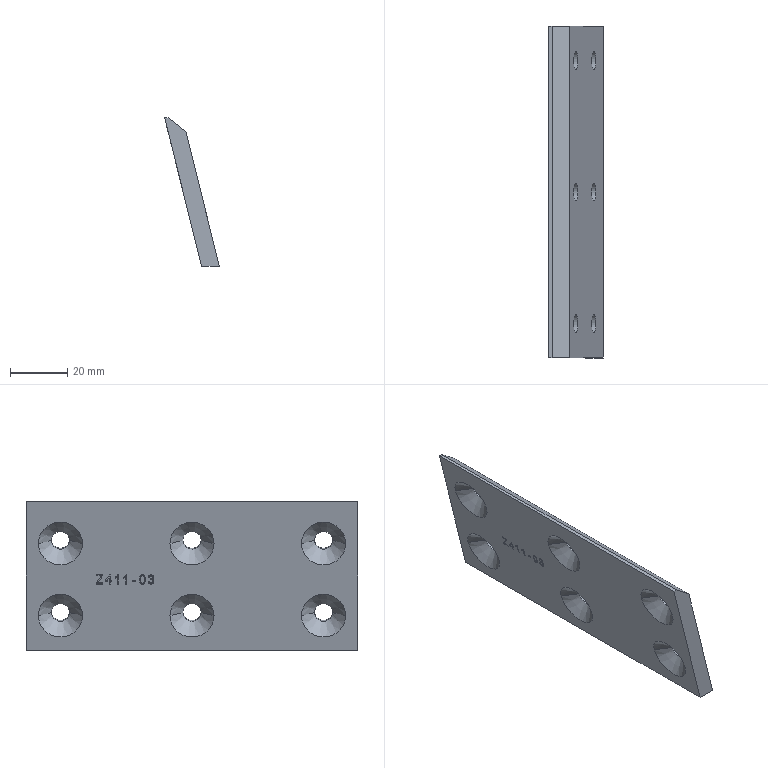Part | Creo | 1 solid | 138 faces | box 19.149 x 116 x 52 mm | volume 32919 mm3 | other 63 | plane 50 | cylinder 13 | cone 12 | commonest cylinder face diameters 6.4 x12 45.582 x1